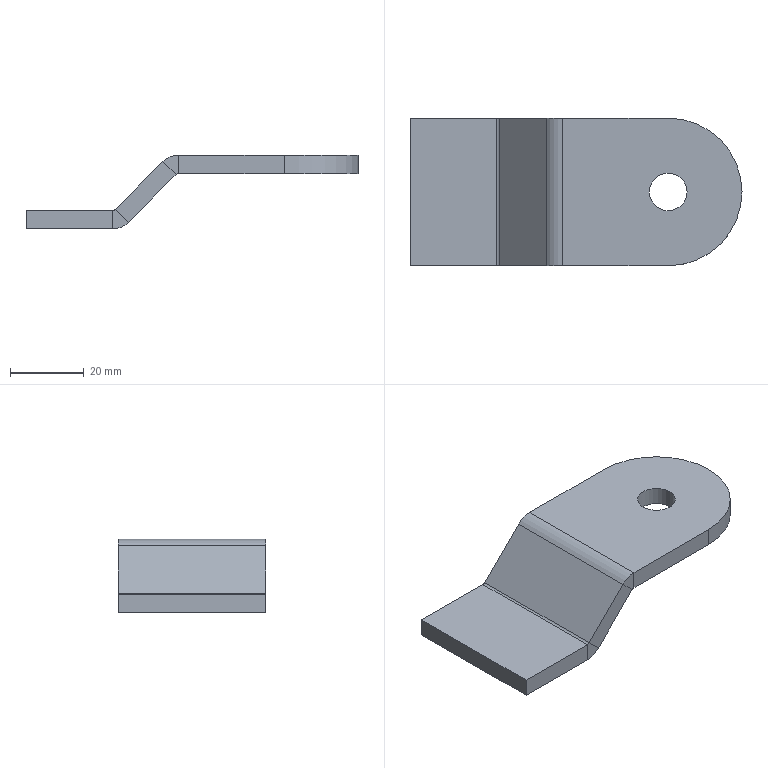Part | STEP file | 5090104 | 1 solid | 23 faces | box 90 x 40 x 20 mm | volume 17915 mm3 | plane 17 | cylinder 6 | commonest cylinder face diameters 2 x2 12 x2 10.2 x1 40 x1
STEP:
#1=CARTESIAN_POINT('',(0.,0.,0.));
#2=DIRECTION('',(0.,0.,1.));
#3=DIRECTION('',(1.,0.,0.));
#4=AXIS2_PLACEMENT_3D('',#1,#2,#3);
#5=CARTESIAN_POINT('',(-42.282,-20.,-13.243));
#6=VERTEX_POINT('',#5);
#7=CARTESIAN_POINT('',(-29.333,-20.,-0.2929));
#8=VERTEX_POINT('',#7);
#9=CARTESIAN_POINT('',(-56.645,-20.,-27.605));
#10=DIRECTION('',(0.7071,0.,0.7071));
#11=VECTOR('',#10,1.);
#12=LINE('',#9,#11);
#13=CARTESIAN_POINT('',(-7.148,0.,21.892));
#14=DIRECTION('',(0.7071,0.,-0.7071));
#15=DIRECTION('',(-0.7071,0.,-0.7071));
#16=AXIS2_PLACEMENT_3D('',#13,#14,#15);
#17=PLANE('',#16);
#18=CARTESIAN_POINT('',(70.,-20.));
#19=DIRECTION('',(-1.,0.));
#20=VECTOR('',#19,1.);
#21=LINE('',#18,#20);
#22=(GEOMETRIC_REPRESENTATION_CONTEXT(2)PARAMETRIC_REPRESENTATION_CONTEXT()REPRESENTATION_CONTEXT('',''));
#23=DEFINITIONAL_REPRESENTATION('',(#21),#22);
#24=PCURVE('',#17,#23);
#25=CARTESIAN_POINT('',(-60.181,-20.,-24.07));
#26=DIRECTION('',(0.,1.,0.));
#27=DIRECTION('',(-0.7071,0.,0.7071));
#28=AXIS2_PLACEMENT_3D('',#25,#26,#27);
#29=PLANE('',#28);
#30=CARTESIAN_POINT('',(-5.,0.));
#31=DIRECTION('',(0.,1.));
#32=VECTOR('',#31,1.);
#33=LINE('',#30,#32);
#34=(GEOMETRIC_REPRESENTATION_CONTEXT(2)PARAMETRIC_REPRESENTATION_CONTEXT()REPRESENTATION_CONTEXT('',''));
#35=DEFINITIONAL_REPRESENTATION('',(#33),#34);
#36=PCURVE('',#29,#35);
#37=SURFACE_CURVE('',#12,(#24,#36),.PCURVE_S1.);
#38=EDGE_CURVE('',#6,#8,#37,.T.);
#39=ORIENTED_EDGE('',*,*,#38,.F.);
#40=CARTESIAN_POINT('',(-42.282,20.,-13.243));
#41=VERTEX_POINT('',#40);
#42=CARTESIAN_POINT('',(-42.282,0.,-13.243));
#43=DIRECTION('',(0.,1.,0.));
#44=VECTOR('',#43,1.);
#45=LINE('',#42,#44);
#46=CARTESIAN_POINT('',(49.688,0.));
#47=DIRECTION('',(0.,1.));
#48=VECTOR('',#47,1.);
#49=LINE('',#46,#48);
#50=(GEOMETRIC_REPRESENTATION_CONTEXT(2)PARAMETRIC_REPRESENTATION_CONTEXT()REPRESENTATION_CONTEXT('',''));
#51=DEFINITIONAL_REPRESENTATION('',(#49),#50);
#52=PCURVE('',#17,#51);
#53=CARTESIAN_POINT('',(-46.525,40.744,-9.));
#54=DIRECTION('',(0.,-1.,0.));
#55=DIRECTION('',(1.,0.,0.));
#56=AXIS2_PLACEMENT_3D('',#53,#54,#55);
#57=CYLINDRICAL_SURFACE('',#56,6.);
#58=CARTESIAN_POINT('',(5.498,40.744));
#59=DIRECTION('',(0.,-1.));
#60=VECTOR('',#59,1.);
#61=LINE('',#58,#60);
#62=(GEOMETRIC_REPRESENTATION_CONTEXT(2)PARAMETRIC_REPRESENTATION_CONTEXT()REPRESENTATION_CONTEXT('',''));
#63=DEFINITIONAL_REPRESENTATION('',(#61),#62);
#64=PCURVE('',#57,#63);
#65=SURFACE_CURVE('',#45,(#52,#64),.PCURVE_S1.);
#66=EDGE_CURVE('',#6,#41,#65,.T.);
#67=ORIENTED_EDGE('',*,*,#66,.T.);
#68=CARTESIAN_POINT('',(-29.333,20.,-0.2929));
#69=VERTEX_POINT('',#68);
#70=CARTESIAN_POINT('',(-56.645,20.,-27.605));
#71=DIRECTION('',(-0.7071,0.,-0.7071));
#72=VECTOR('',#71,1.);
#73=LINE('',#70,#72);
#74=CARTESIAN_POINT('',(70.,20.));
#75=DIRECTION('',(1.,0.));
#76=VECTOR('',#75,1.);
#77=LINE('',#74,#76);
#78=(GEOMETRIC_REPRESENTATION_CONTEXT(2)PARAMETRIC_REPRESENTATION_CONTEXT()REPRESENTATION_CONTEXT('',''));
#79=DEFINITIONAL_REPRESENTATION('',(#77),#78);
#80=PCURVE('',#17,#79);
#81=CARTESIAN_POINT('',(-60.181,20.,-24.07));
#82=DIRECTION('',(0.,-1.,0.));
#83=DIRECTION('',(0.7071,0.,-0.7071));
#84=AXIS2_PLACEMENT_3D('',#81,#82,#83);
#85=PLANE('',#84);
#86=CARTESIAN_POINT('',(5.,0.));
#87=DIRECTION('',(0.,-1.));
#88=VECTOR('',#87,1.);
#89=LINE('',#86,#88);
#90=(GEOMETRIC_REPRESENTATION_CONTEXT(2)PARAMETRIC_REPRESENTATION_CONTEXT()REPRESENTATION_CONTEXT('',''));
#91=DEFINITIONAL_REPRESENTATION('',(#89),#90);
#92=PCURVE('',#85,#91);
#93=SURFACE_CURVE('',#73,(#80,#92),.PCURVE_S1.);
#94=EDGE_CURVE('',#69,#41,#93,.T.);
#95=ORIENTED_EDGE('',*,*,#94,.F.);
#96=CARTESIAN_POINT('',(-29.333,0.,-0.2929));
#97=DIRECTION('',(0.,1.,0.));
#98=VECTOR('',#97,1.);
#99=LINE('',#96,#98);
#100=CARTESIAN_POINT('',(31.374,0.));
#101=DIRECTION('',(0.,1.));
#102=VECTOR('',#101,1.);
#103=LINE('',#100,#102);
#104=(GEOMETRIC_REPRESENTATION_CONTEXT(2)PARAMETRIC_REPRESENTATION_CONTEXT()REPRESENTATION_CONTEXT('',''));
#105=DEFINITIONAL_REPRESENTATION('',(#103),#104);
#106=PCURVE('',#17,#105);
#107=CARTESIAN_POINT('',(-28.626,40.405,-1.));
#108=DIRECTION('',(0.,-1.,0.));
#109=DIRECTION('',(1.,0.,0.));
#110=AXIS2_PLACEMENT_3D('',#107,#108,#109);
#111=CYLINDRICAL_SURFACE('',#110,1.);
#112=CARTESIAN_POINT('',(2.356,40.405));
#113=DIRECTION('',(0.,-1.));
#114=VECTOR('',#113,1.);
#115=LINE('',#112,#114);
#116=(GEOMETRIC_REPRESENTATION_CONTEXT(2)PARAMETRIC_REPRESENTATION_CONTEXT()REPRESENTATION_CONTEXT('',''));
#117=DEFINITIONAL_REPRESENTATION('',(#115),#116);
#118=PCURVE('',#111,#117);
#119=SURFACE_CURVE('',#99,(#106,#118),.PCURVE_S1.);
#120=EDGE_CURVE('',#8,#69,#119,.T.);
#121=ORIENTED_EDGE('',*,*,#120,.F.);
#122=EDGE_LOOP('',(#39,#67,#95,#121));
#123=FACE_BOUND('',#122,.T.);
#124=ADVANCED_FACE('',(#123),#17,.T.);
#125=CARTESIAN_POINT('',(-45.818,20.,-9.707));
#126=VERTEX_POINT('',#125);
#127=CARTESIAN_POINT('',(-45.818,20.,-9.707));
#128=DIRECTION('',(0.7071,0.,-0.7071));
#129=VECTOR('',#128,1.);
#130=LINE('',#127,#129);
#131=CARTESIAN_POINT('',(0.,20.312));
#132=DIRECTION('',(1.,0.));
#133=VECTOR('',#132,1.);
#134=LINE('',#131,#133);
#135=(GEOMETRIC_REPRESENTATION_CONTEXT(2)PARAMETRIC_REPRESENTATION_CONTEXT()REPRESENTATION_CONTEXT('',''));
#136=DEFINITIONAL_REPRESENTATION('',(#134),#135);
#137=PCURVE('',#85,#136);
#138=CARTESIAN_POINT('',(-46.525,20.,-9.));
#139=DIRECTION('',(0.,-1.,0.));
#140=DIRECTION('',(0.,0.,-1.));
#141=AXIS2_PLACEMENT_3D('',#138,#139,#140);
#142=PLANE('',#141);
#143=CARTESIAN_POINT('',(0.7071,0.7071));
#144=DIRECTION('',(0.7071,0.7071));
#145=VECTOR('',#144,1.);
#146=LINE('',#143,#145);
#147=(GEOMETRIC_REPRESENTATION_CONTEXT(2)PARAMETRIC_REPRESENTATION_CONTEXT()REPRESENTATION_CONTEXT('',''));
#148=DEFINITIONAL_REPRESENTATION('',(#146),#147);
#149=PCURVE('',#142,#148);
#150=SURFACE_CURVE('',#130,(#137,#149),.PCURVE_S1.);
#151=EDGE_CURVE('',#126,#41,#150,.T.);
#152=ORIENTED_EDGE('',*,*,#151,.F.);
#153=CARTESIAN_POINT('',(-32.868,20.,3.243));
#154=VERTEX_POINT('',#153);
#155=CARTESIAN_POINT('',(-60.181,20.,-24.07));
#156=DIRECTION('',(-0.7071,0.,-0.7071));
#157=VECTOR('',#156,1.);
#158=LINE('',#155,#157);
#159=CARTESIAN_POINT('',(0.,0.));
#160=DIRECTION('',(0.,-1.));
#161=VECTOR('',#160,1.);
#162=LINE('',#159,#161);
#163=(GEOMETRIC_REPRESENTATION_CONTEXT(2)PARAMETRIC_REPRESENTATION_CONTEXT()REPRESENTATION_CONTEXT('',''));
#164=DEFINITIONAL_REPRESENTATION('',(#162),#163);
#165=PCURVE('',#85,#164);
#166=CARTESIAN_POINT('',(-10.683,0.,25.428));
#167=DIRECTION('',(0.7071,0.,-0.7071));
#168=DIRECTION('',(-0.7071,0.,-0.7071));
#169=AXIS2_PLACEMENT_3D('',#166,#167,#168);
#170=PLANE('',#169);
#171=CARTESIAN_POINT('',(70.,20.));
#172=DIRECTION('',(1.,0.));
#173=VECTOR('',#172,1.);
#174=LINE('',#171,#173);
#175=(GEOMETRIC_REPRESENTATION_CONTEXT(2)PARAMETRIC_REPRESENTATION_CONTEXT()REPRESENTATION_CONTEXT('',''));
#176=DEFINITIONAL_REPRESENTATION('',(#174),#175);
#177=PCURVE('',#170,#176);
#178=SURFACE_CURVE('',#158,(#165,#177),.PCURVE_S1.);
#179=EDGE_CURVE('',#154,#126,#178,.T.);
#180=ORIENTED_EDGE('',*,*,#179,.F.);
#181=CARTESIAN_POINT('',(-32.868,20.,3.243));
#182=DIRECTION('',(0.7071,0.,-0.7071));
#183=VECTOR('',#182,1.);
#184=LINE('',#181,#183);
#185=CARTESIAN_POINT('',(0.,38.626));
#186=DIRECTION('',(1.,0.));
#187=VECTOR('',#186,1.);
#188=LINE('',#185,#187);
#189=(GEOMETRIC_REPRESENTATION_CONTEXT(2)PARAMETRIC_REPRESENTATION_CONTEXT()REPRESENTATION_CONTEXT('',''));
#190=DEFINITIONAL_REPRESENTATION('',(#188),#189);
#191=PCURVE('',#85,#190);
#192=CARTESIAN_POINT('',(-28.626,20.,-1.));
#193=DIRECTION('',(0.,1.,0.));
#194=DIRECTION('',(0.,0.,1.));
#195=AXIS2_PLACEMENT_3D('',#192,#193,#194);
#196=PLANE('',#195);
#197=CARTESIAN_POINT('',(4.243,-4.243));
#198=DIRECTION('',(-0.7071,0.7071));
#199=VECTOR('',#198,1.);
#200=LINE('',#197,#199);
#201=(GEOMETRIC_REPRESENTATION_CONTEXT(2)PARAMETRIC_REPRESENTATION_CONTEXT()REPRESENTATION_CONTEXT('',''));
#202=DEFINITIONAL_REPRESENTATION('',(#200),#201);
#203=PCURVE('',#196,#202);
#204=SURFACE_CURVE('',#184,(#191,#203),.PCURVE_S1.);
#205=EDGE_CURVE('',#154,#69,#204,.T.);
#206=ORIENTED_EDGE('',*,*,#205,.T.);
#207=ORIENTED_EDGE('',*,*,#94,.T.);
#208=EDGE_LOOP('',(#152,#180,#206,#207));
#209=FACE_BOUND('',#208,.T.);
#210=ADVANCED_FACE('',(#209),#85,.F.);
#211=CARTESIAN_POINT('',(-45.818,-20.,-9.707));
#212=VERTEX_POINT('',#211);
#213=CARTESIAN_POINT('',(-45.818,-20.,-9.707));
#214=DIRECTION('',(-0.7071,0.,0.7071));
#215=VECTOR('',#214,1.);
#216=LINE('',#213,#215);
#217=CARTESIAN_POINT('',(0.,20.312));
#218=DIRECTION('',(1.,0.));
#219=VECTOR('',#218,1.);
#220=LINE('',#217,#219);
#221=(GEOMETRIC_REPRESENTATION_CONTEXT(2)PARAMETRIC_REPRESENTATION_CONTEXT()REPRESENTATION_CONTEXT('',''));
#222=DEFINITIONAL_REPRESENTATION('',(#220),#221);
#223=PCURVE('',#29,#222);
#224=CARTESIAN_POINT('',(-46.525,-20.,-9.));
#225=DIRECTION('',(0.,1.,0.));
#226=DIRECTION('',(0.,0.,1.));
#227=AXIS2_PLACEMENT_3D('',#224,#225,#226);
#228=PLANE('',#227);
#229=CARTESIAN_POINT('',(-0.7071,0.7071));
#230=DIRECTION('',(0.7071,-0.7071));
#231=VECTOR('',#230,1.);
#232=LINE('',#229,#231);
#233=(GEOMETRIC_REPRESENTATION_CONTEXT(2)PARAMETRIC_REPRESENTATION_CONTEXT()REPRESENTATION_CONTEXT('',''));
#234=DEFINITIONAL_REPRESENTATION('',(#232),#233);
#235=PCURVE('',#228,#234);
#236=SURFACE_CURVE('',#216,(#223,#235),.PCURVE_S1.);
#237=EDGE_CURVE('',#6,#212,#236,.T.);
#238=ORIENTED_EDGE('',*,*,#237,.F.);
#239=ORIENTED_EDGE('',*,*,#38,.T.);
#240=CARTESIAN_POINT('',(-32.868,-20.,3.243));
#241=VERTEX_POINT('',#240);
#242=CARTESIAN_POINT('',(-32.868,-20.,3.243));
#243=DIRECTION('',(-0.7071,0.,0.7071));
#244=VECTOR('',#243,1.);
#245=LINE('',#242,#244);
#246=CARTESIAN_POINT('',(0.,38.626));
#247=DIRECTION('',(1.,0.));
#248=VECTOR('',#247,1.);
#249=LINE('',#246,#248);
#250=(GEOMETRIC_REPRESENTATION_CONTEXT(2)PARAMETRIC_REPRESENTATION_CONTEXT()REPRESENTATION_CONTEXT('',''));
#251=DEFINITIONAL_REPRESENTATION('',(#249),#250);
#252=PCURVE('',#29,#251);
#253=CARTESIAN_POINT('',(-28.626,-20.,-1.));
#254=DIRECTION('',(0.,-1.,0.));
#255=DIRECTION('',(0.,0.,-1.));
#256=AXIS2_PLACEMENT_3D('',#253,#254,#255);
#257=PLANE('',#256);
#258=CARTESIAN_POINT('',(-4.243,-4.243));
#259=DIRECTION('',(-0.7071,-0.7071));
#260=VECTOR('',#259,1.);
#261=LINE('',#258,#260);
#262=(GEOMETRIC_REPRESENTATION_CONTEXT(2)PARAMETRIC_REPRESENTATION_CONTEXT()REPRESENTATION_CONTEXT('',''));
#263=DEFINITIONAL_REPRESENTATION('',(#261),#262);
#264=PCURVE('',#257,#263);
#265=SURFACE_CURVE('',#245,(#252,#264),.PCURVE_S1.);
#266=EDGE_CURVE('',#8,#241,#265,.T.);
#267=ORIENTED_EDGE('',*,*,#266,.T.);
#268=CARTESIAN_POINT('',(-60.181,-20.,-24.07));
#269=DIRECTION('',(0.7071,0.,0.7071));
#270=VECTOR('',#269,1.);
#271=LINE('',#268,#270);
#272=CARTESIAN_POINT('',(0.,0.));
#273=DIRECTION('',(0.,1.));
#274=VECTOR('',#273,1.);
#275=LINE('',#272,#274);
#276=(GEOMETRIC_REPRESENTATION_CONTEXT(2)PARAMETRIC_REPRESENTATION_CONTEXT()REPRESENTATION_CONTEXT('',''));
#277=DEFINITIONAL_REPRESENTATION('',(#275),#276);
#278=PCURVE('',#29,#277);
#279=CARTESIAN_POINT('',(70.,-20.));
#280=DIRECTION('',(-1.,0.));
#281=VECTOR('',#280,1.);
#282=LINE('',#279,#281);
#283=(GEOMETRIC_REPRESENTATION_CONTEXT(2)PARAMETRIC_REPRESENTATION_CONTEXT()REPRESENTATION_CONTEXT('',''));
#284=DEFINITIONAL_REPRESENTATION('',(#282),#283);
#285=PCURVE('',#170,#284);
#286=SURFACE_CURVE('',#271,(#278,#285),.PCURVE_S1.);
#287=EDGE_CURVE('',#212,#241,#286,.T.);
#288=ORIENTED_EDGE('',*,*,#287,.F.);
#289=EDGE_LOOP('',(#238,#239,#267,#288));
#290=FACE_BOUND('',#289,.T.);
#291=ADVANCED_FACE('',(#290),#29,.F.);
#292=CARTESIAN_POINT('',(-45.818,0.,-9.707));
#293=DIRECTION('',(0.,1.,0.));
#294=VECTOR('',#293,1.);
#295=LINE('',#292,#294);
#296=CARTESIAN_POINT('',(49.688,0.));
#297=DIRECTION('',(0.,1.));
#298=VECTOR('',#297,1.);
#299=LINE('',#296,#298);
#300=(GEOMETRIC_REPRESENTATION_CONTEXT(2)PARAMETRIC_REPRESENTATION_CONTEXT()REPRESENTATION_CONTEXT('',''));
#301=DEFINITIONAL_REPRESENTATION('',(#299),#300);
#302=PCURVE('',#170,#301);
#303=CARTESIAN_POINT('',(-46.525,40.744,-9.));
#304=DIRECTION('',(0.,-1.,0.));
#305=DIRECTION('',(1.,0.,0.));
#306=AXIS2_PLACEMENT_3D('',#303,#304,#305);
#307=CYLINDRICAL_SURFACE('',#306,1.);
#308=CARTESIAN_POINT('',(5.498,40.744));
#309=DIRECTION('',(0.,-1.));
#310=VECTOR('',#309,1.);
#311=LINE('',#308,#310);
#312=(GEOMETRIC_REPRESENTATION_CONTEXT(2)PARAMETRIC_REPRESENTATION_CONTEXT()REPRESENTATION_CONTEXT('',''));
#313=DEFINITIONAL_REPRESENTATION('',(#311),#312);
#314=PCURVE('',#307,#313);
#315=SURFACE_CURVE('',#295,(#302,#314),.PCURVE_S1.);
#316=EDGE_CURVE('',#212,#126,#315,.T.);
#317=ORIENTED_EDGE('',*,*,#316,.F.);
#318=ORIENTED_EDGE('',*,*,#287,.T.);
#319=CARTESIAN_POINT('',(-32.868,0.,3.243));
#320=DIRECTION('',(0.,1.,0.));
#321=VECTOR('',#320,1.);
#322=LINE('',#319,#321);
#323=CARTESIAN_POINT('',(31.374,0.));
#324=DIRECTION('',(0.,1.));
#325=VECTOR('',#324,1.);
#326=LINE('',#323,#325);
#327=(GEOMETRIC_REPRESENTATION_CONTEXT(2)PARAMETRIC_REPRESENTATION_CONTEXT()REPRESENTATION_CONTEXT('',''));
#328=DEFINITIONAL_REPRESENTATION('',(#326),#327);
#329=PCURVE('',#170,#328);
#330=CARTESIAN_POINT('',(-28.626,40.405,-1.));
#331=DIRECTION('',(0.,-1.,0.));
#332=DIRECTION('',(1.,0.,0.));
#333=AXIS2_PLACEMENT_3D('',#330,#331,#332);
#334=CYLINDRICAL_SURFACE('',#333,6.);
#335=CARTESIAN_POINT('',(2.356,40.405));
#336=DIRECTION('',(0.,-1.));
#337=VECTOR('',#336,1.);
#338=LINE('',#335,#337);
#339=(GEOMETRIC_REPRESENTATION_CONTEXT(2)PARAMETRIC_REPRESENTATION_CONTEXT()REPRESENTATION_CONTEXT('',''));
#340=DEFINITIONAL_REPRESENTATION('',(#338),#339);
#341=PCURVE('',#334,#340);
#342=SURFACE_CURVE('',#322,(#329,#341),.PCURVE_S1.);
#343=EDGE_CURVE('',#241,#154,#342,.T.);
#344=ORIENTED_EDGE('',*,*,#343,.T.);
#345=ORIENTED_EDGE('',*,*,#179,.T.);
#346=EDGE_LOOP('',(#317,#318,#344,#345));
#347=FACE_BOUND('',#346,.T.);
#348=ADVANCED_FACE('',(#347),#170,.F.);
#349=CARTESIAN_POINT('',(5.1,0.,5.));
#350=VERTEX_POINT('',#349);
#351=CARTESIAN_POINT('',(0.,0.,5.));
#352=DIRECTION('',(0.,0.,1.));
#353=DIRECTION('',(1.,0.,0.));
#354=AXIS2_PLACEMENT_3D('',#351,#352,#353);
#355=CIRCLE('',#354,5.1);
#356=CARTESIAN_POINT('',(0.,0.,5.));
#357=DIRECTION('',(0.,0.,-1.));
#358=DIRECTION('',(-1.,0.,0.));
#359=AXIS2_PLACEMENT_3D('',#356,#357,#358);
#360=CYLINDRICAL_SURFACE('',#359,5.1);
#361=CARTESIAN_POINT('',(9.425,0.));
#362=DIRECTION('',(-1.,0.));
#363=VECTOR('',#362,1.);
#364=LINE('',#361,#363);
#365=(GEOMETRIC_REPRESENTATION_CONTEXT(2)PARAMETRIC_REPRESENTATION_CONTEXT()REPRESENTATION_CONTEXT('',''));
#366=DEFINITIONAL_REPRESENTATION('',(#364),#365);
#367=PCURVE('',#360,#366);
#368=CARTESIAN_POINT('',(0.,0.,5.));
#369=DIRECTION('',(0.,0.,-1.));
#370=DIRECTION('',(-1.,0.,0.));
#371=AXIS2_PLACEMENT_3D('',#368,#369,#370);
#372=PLANE('',#371);
#373=CARTESIAN_POINT('',(-5.1,0.));
#374=CARTESIAN_POINT('',(-5.1,8.833));
#375=CARTESIAN_POINT('',(2.55,4.417));
#376=CARTESIAN_POINT('',(10.2,0.));
#377=CARTESIAN_POINT('',(2.55,-4.417));
#378=CARTESIAN_POINT('',(-5.1,-8.833));
#379=CARTESIAN_POINT('',(-5.1,0.));
#380=(BOUNDED_CURVE()B_SPLINE_CURVE(2,(#373,#374,#375,#376,#377,#378,#379),.UNSPECIFIED.,.T.,.F.)B_SPLINE_CURVE_WITH_KNOTS((1,2,2,2,2,1),(-2.094,0.,2.094,4.189,6.283,8.378),.UNSPECIFIED.)CURVE()GEOMETRIC_REPRESENTATION_ITEM()RATIONAL_B_SPLINE_CURVE((1.,0.5,1.,0.5,1.,0.5,1.))REPRESENTATION_ITEM(''));
#381=(GEOMETRIC_REPRESENTATION_CONTEXT(2)PARAMETRIC_REPRESENTATION_CONTEXT()REPRESENTATION_CONTEXT('',''));
#382=DEFINITIONAL_REPRESENTATION('',(#380),#381);
#383=PCURVE('',#372,#382);
#384=SURFACE_CURVE('',#355,(#367,#383),.PCURVE_S1.);
#385=EDGE_CURVE('',#350,#350,#384,.T.);
#386=ORIENTED_EDGE('',*,*,#385,.F.);
#387=CARTESIAN_POINT('',(5.1,0.,0.));
#388=VERTEX_POINT('',#387);
#389=CARTESIAN_POINT('',(5.1,0.,5.));
#390=CARTESIAN_POINT('',(5.1,0.,0.));
#391=B_SPLINE_CURVE_WITH_KNOTS('',1,(#389,#390),.UNSPECIFIED.,.F.,.F.,(2,2),(0.,5.),.PIECEWISE_BEZIER_KNOTS.);
#392=CARTESIAN_POINT('',(9.425,0.));
#393=DIRECTION('',(0.,1.));
#394=VECTOR('',#393,1.);
#395=LINE('',#392,#394);
#396=(GEOMETRIC_REPRESENTATION_CONTEXT(2)PARAMETRIC_REPRESENTATION_CONTEXT()REPRESENTATION_CONTEXT('',''));
#397=DEFINITIONAL_REPRESENTATION('',(#395),#396);
#398=PCURVE('',#360,#397);
#399=CARTESIAN_POINT('',(3.142,0.));
#400=DIRECTION('',(0.,1.));
#401=VECTOR('',#400,1.);
#402=LINE('',#399,#401);
#403=(GEOMETRIC_REPRESENTATION_CONTEXT(2)PARAMETRIC_REPRESENTATION_CONTEXT()REPRESENTATION_CONTEXT('',''));
#404=DEFINITIONAL_REPRESENTATION('',(#402),#403);
#405=PCURVE('',#360,#404);
#406=SEAM_CURVE('',#391,(#398,#405),.PCURVE_S1.);
#407=EDGE_CURVE('',#350,#388,#406,.T.);
#408=ORIENTED_EDGE('',*,*,#407,.T.);
#409=CARTESIAN_POINT('',(0.,0.,0.));
#410=DIRECTION('',(0.,0.,1.));
#411=DIRECTION('',(1.,0.,0.));
#412=AXIS2_PLACEMENT_3D('',#409,#410,#411);
#413=CIRCLE('',#412,5.1);
#414=CARTESIAN_POINT('',(9.425,5.));
#415=DIRECTION('',(-1.,0.));
#416=VECTOR('',#415,1.);
#417=LINE('',#414,#416);
#418=(GEOMETRIC_REPRESENTATION_CONTEXT(2)PARAMETRIC_REPRESENTATION_CONTEXT()REPRESENTATION_CONTEXT('',''));
#419=DEFINITIONAL_REPRESENTATION('',(#417),#418);
#420=PCURVE('',#360,#419);
#421=CARTESIAN_POINT('',(0.,0.,0.));
#422=DIRECTION('',(0.,0.,-1.));
#423=DIRECTION('',(-1.,0.,0.));
#424=AXIS2_PLACEMENT_3D('',#421,#422,#423);
#425=PLANE('',#424);
#426=CARTESIAN_POINT('',(-5.1,0.));
#427=CARTESIAN_POINT('',(-5.1,8.833));
#428=CARTESIAN_POINT('',(2.55,4.417));
#429=CARTESIAN_POINT('',(10.2,0.));
#430=CARTESIAN_POINT('',(2.55,-4.417));
#431=CARTESIAN_POINT('',(-5.1,-8.833));
#432=CARTESIAN_POINT('',(-5.1,0.));
#433=(BOUNDED_CURVE()B_SPLINE_CURVE(2,(#426,#427,#428,#429,#430,#431,#432),.UNSPECIFIED.,.T.,.F.)B_SPLINE_CURVE_WITH_KNOTS((1,2,2,2,2,1),(-2.094,0.,2.094,4.189,6.283,8.378),.UNSPECIFIED.)CURVE()GEOMETRIC_REPRESENTATION_ITEM()RATIONAL_B_SPLINE_CURVE((1.,0.5,1.,0.5,1.,0.5,1.))REPRESENTATION_ITEM(''));
#434=(GEOMETRIC_REPRESENTATION_CONTEXT(2)PARAMETRIC_REPRESENTATION_CONTEXT()REPRESENTATION_CONTEXT('',''));
#435=DEFINITIONAL_REPRESENTATION('',(#433),#434);
#436=PCURVE('',#425,#435);
#437=SURFACE_CURVE('',#413,(#420,#436),.PCURVE_S1.);
#438=EDGE_CURVE('',#388,#388,#437,.T.);
#439=ORIENTED_EDGE('',*,*,#438,.T.);
#440=ORIENTED_EDGE('',*,*,#407,.F.);
#441=EDGE_LOOP('',(#386,#408,#439,#440));
#442=FACE_BOUND('',#441,.F.);
#443=ADVANCED_FACE('',(#442),#360,.F.);
#444=CARTESIAN_POINT('',(0.,-20.,0.));
#445=VERTEX_POINT('',#444);
#446=CARTESIAN_POINT('',(0.,20.,0.));
#447=VERTEX_POINT('',#446);
#448=CARTESIAN_POINT('',(0.,0.,0.));
#449=DIRECTION('',(0.,0.,1.));
#450=DIRECTION('',(-1.,0.,0.));
#451=AXIS2_PLACEMENT_3D('',#448,#449,#450);
#452=CIRCLE('',#451,20.);
#453=CARTESIAN_POINT('',(0.,0.,5.));
#454=DIRECTION('',(0.,0.,-1.));
#455=DIRECTION('',(-1.,0.,0.));
#456=AXIS2_PLACEMENT_3D('',#453,#454,#455);
#457=CYLINDRICAL_SURFACE('',#456,20.);
#458=CARTESIAN_POINT('',(6.283,5.));
#459=DIRECTION('',(-1.,0.));
#460=VECTOR('',#459,1.);
#461=LINE('',#458,#460);
#462=(GEOMETRIC_REPRESENTATION_CONTEXT(2)PARAMETRIC_REPRESENTATION_CONTEXT()REPRESENTATION_CONTEXT('',''));
#463=DEFINITIONAL_REPRESENTATION('',(#461),#462);
#464=PCURVE('',#457,#463);
#465=CARTESIAN_POINT('',(20.,0.));
#466=CARTESIAN_POINT('',(20.,-34.641));
#467=CARTESIAN_POINT('',(-10.,-17.321));
#468=CARTESIAN_POINT('',(-40.,0.));
#469=CARTESIAN_POINT('',(-10.,17.321));
#470=CARTESIAN_POINT('',(20.,34.641));
#471=CARTESIAN_POINT('',(20.,0.));
#472=(BOUNDED_CURVE()B_SPLINE_CURVE(2,(#465,#466,#467,#468,#469,#470,#471),.UNSPECIFIED.,.T.,.F.)B_SPLINE_CURVE_WITH_KNOTS((1,2,2,2,2,1),(-2.094,0.,2.094,4.189,6.283,8.378),.UNSPECIFIED.)CURVE()GEOMETRIC_REPRESENTATION_ITEM()RATIONAL_B_SPLINE_CURVE((1.,0.5,1.,0.5,1.,0.5,1.))REPRESENTATION_ITEM(''));
#473=(GEOMETRIC_REPRESENTATION_CONTEXT(2)PARAMETRIC_REPRESENTATION_CONTEXT()REPRESENTATION_CONTEXT('',''));
#474=DEFINITIONAL_REPRESENTATION('',(#472),#473);
#475=PCURVE('',#425,#474);
#476=SURFACE_CURVE('',#452,(#464,#475),.PCURVE_S1.);
#477=EDGE_CURVE('',#445,#447,#476,.T.);
#478=ORIENTED_EDGE('',*,*,#477,.T.);
#479=CARTESIAN_POINT('',(0.,20.,5.));
#480=VERTEX_POINT('',#479);
#481=CARTESIAN_POINT('',(0.,20.,5.));
#482=DIRECTION('',(0.,0.,-1.));
#483=VECTOR('',#482,1.);
#484=LINE('',#481,#483);
#485=CARTESIAN_POINT('',(1.571,0.));
#486=DIRECTION('',(0.,1.));
#487=VECTOR('',#486,1.);
#488=LINE('',#485,#487);
#489=(GEOMETRIC_REPRESENTATION_CONTEXT(2)PARAMETRIC_REPRESENTATION_CONTEXT()REPRESENTATION_CONTEXT('',''));
#490=DEFINITIONAL_REPRESENTATION('',(#488),#489);
#491=PCURVE('',#457,#490);
#492=CARTESIAN_POINT('',(-70.,20.,5.));
#493=DIRECTION('',(0.,-1.,0.));
#494=DIRECTION('',(0.,0.,-1.));
#495=AXIS2_PLACEMENT_3D('',#492,#493,#494);
#496=PLANE('',#495);
#497=CARTESIAN_POINT('',(0.,70.));
#498=DIRECTION('',(1.,0.));
#499=VECTOR('',#498,1.);
#500=LINE('',#497,#499);
#501=(GEOMETRIC_REPRESENTATION_CONTEXT(2)PARAMETRIC_REPRESENTATION_CONTEXT()REPRESENTATION_CONTEXT('',''));
#502=DEFINITIONAL_REPRESENTATION('',(#500),#501);
#503=PCURVE('',#496,#502);
#504=SURFACE_CURVE('',#484,(#491,#503),.PCURVE_S1.);
#505=EDGE_CURVE('',#480,#447,#504,.T.);
#506=ORIENTED_EDGE('',*,*,#505,.F.);
#507=CARTESIAN_POINT('',(0.,-20.,5.));
#508=VERTEX_POINT('',#507);
#509=CARTESIAN_POINT('',(0.,0.,5.));
#510=DIRECTION('',(0.,0.,1.));
#511=DIRECTION('',(-1.,0.,0.));
#512=AXIS2_PLACEMENT_3D('',#509,#510,#511);
#513=CIRCLE('',#512,20.);
#514=CARTESIAN_POINT('',(6.283,0.));
#515=DIRECTION('',(-1.,0.));
#516=VECTOR('',#515,1.);
#517=LINE('',#514,#516);
#518=(GEOMETRIC_REPRESENTATION_CONTEXT(2)PARAMETRIC_REPRESENTATION_CONTEXT()REPRESENTATION_CONTEXT('',''));
#519=DEFINITIONAL_REPRESENTATION('',(#517),#518);
#520=PCURVE('',#457,#519);
#521=CARTESIAN_POINT('',(20.,0.));
#522=CARTESIAN_POINT('',(20.,-34.641));
#523=CARTESIAN_POINT('',(-10.,-17.321));
#524=CARTESIAN_POINT('',(-40.,0.));
#525=CARTESIAN_POINT('',(-10.,17.321));
#526=CARTESIAN_POINT('',(20.,34.641));
#527=CARTESIAN_POINT('',(20.,0.));
#528=(BOUNDED_CURVE()B_SPLINE_CURVE(2,(#521,#522,#523,#524,#525,#526,#527),.UNSPECIFIED.,.T.,.F.)B_SPLINE_CURVE_WITH_KNOTS((1,2,2,2,2,1),(-2.094,0.,2.094,4.189,6.283,8.378),.UNSPECIFIED.)CURVE()GEOMETRIC_REPRESENTATION_ITEM()RATIONAL_B_SPLINE_CURVE((1.,0.5,1.,0.5,1.,0.5,1.))REPRESENTATION_ITEM(''));
#529=(GEOMETRIC_REPRESENTATION_CONTEXT(2)PARAMETRIC_REPRESENTATION_CONTEXT()REPRESENTATION_CONTEXT('',''));
#530=DEFINITIONAL_REPRESENTATION('',(#528),#529);
#531=PCURVE('',#372,#530);
#532=SURFACE_CURVE('',#513,(#520,#531),.PCURVE_S1.);
#533=EDGE_CURVE('',#508,#480,#532,.T.);
#534=ORIENTED_EDGE('',*,*,#533,.F.);
#535=CARTESIAN_POINT('',(0.,-20.,5.));
#536=DIRECTION('',(0.,0.,-1.));
#537=VECTOR('',#536,1.);
#538=LINE('',#535,#537);
#539=CARTESIAN_POINT('',(4.712,0.));
#540=DIRECTION('',(0.,1.));
#541=VECTOR('',#540,1.);
#542=LINE('',#539,#541);
#543=(GEOMETRIC_REPRESENTATION_CONTEXT(2)PARAMETRIC_REPRESENTATION_CONTEXT()REPRESENTATION_CONTEXT('',''));
#544=DEFINITIONAL_REPRESENTATION('',(#542),#543);
#545=PCURVE('',#457,#544);
#546=CARTESIAN_POINT('',(-70.,-20.,5.));
#547=DIRECTION('',(0.,1.,0.));
#548=DIRECTION('',(0.,0.,1.));
#549=AXIS2_PLACEMENT_3D('',#546,#547,#548);
#550=PLANE('',#549);
#551=CARTESIAN_POINT('',(0.,70.));
#552=DIRECTION('',(-1.,0.));
#553=VECTOR('',#552,1.);
#554=LINE('',#551,#553);
#555=(GEOMETRIC_REPRESENTATION_CONTEXT(2)PARAMETRIC_REPRESENTATION_CONTEXT()REPRESENTATION_CONTEXT('',''));
#556=DEFINITIONAL_REPRESENTATION('',(#554),#555);
#557=PCURVE('',#550,#556);
#558=SURFACE_CURVE('',#538,(#545,#557),.PCURVE_S1.);
#559=EDGE_CURVE('',#508,#445,#558,.T.);
#560=ORIENTED_EDGE('',*,*,#559,.T.);
#561=EDGE_LOOP('',(#478,#506,#534,#560));
#562=FACE_BOUND('',#561,.T.);
#563=ADVANCED_FACE('',(#562),#457,.T.);
#564=CARTESIAN_POINT('',(-28.626,-20.,5.));
#565=VERTEX_POINT('',#564);
#566=CARTESIAN_POINT('',(-28.626,20.,5.));
#567=VERTEX_POINT('',#566);
#568=CARTESIAN_POINT('',(-28.626,0.,5.));
#569=DIRECTION('',(0.,1.,0.));
#570=VECTOR('',#569,1.);
#571=LINE('',#568,#570);
#572=CARTESIAN_POINT('',(28.626,0.));
#573=DIRECTION('',(0.,1.));
#574=VECTOR('',#573,1.);
#575=LINE('',#572,#574);
#576=(GEOMETRIC_REPRESENTATION_CONTEXT(2)PARAMETRIC_REPRESENTATION_CONTEXT()REPRESENTATION_CONTEXT('',''));
#577=DEFINITIONAL_REPRESENTATION('',(#575),#576);
#578=PCURVE('',#372,#577);
#579=CARTESIAN_POINT('',(1.571,40.405));
#580=DIRECTION('',(0.,-1.));
#581=VECTOR('',#580,1.);
#582=LINE('',#579,#581);
#583=(GEOMETRIC_REPRESENTATION_CONTEXT(2)PARAMETRIC_REPRESENTATION_CONTEXT()REPRESENTATION_CONTEXT('',''));
#584=DEFINITIONAL_REPRESENTATION('',(#582),#583);
#585=PCURVE('',#334,#584);
#586=SURFACE_CURVE('',#571,(#578,#585),.PCURVE_S1.);
#587=EDGE_CURVE('',#565,#567,#586,.T.);
#588=ORIENTED_EDGE('',*,*,#587,.F.);
#589=CARTESIAN_POINT('',(-70.,-20.,5.));
#590=DIRECTION('',(1.,0.,0.));
#591=VECTOR('',#590,1.);
#592=LINE('',#589,#591);
#593=CARTESIAN_POINT('',(70.,-20.));
#594=DIRECTION('',(-1.,0.));
#595=VECTOR('',#594,1.);
#596=LINE('',#593,#595);
#597=(GEOMETRIC_REPRESENTATION_CONTEXT(2)PARAMETRIC_REPRESENTATION_CONTEXT()REPRESENTATION_CONTEXT('',''));
#598=DEFINITIONAL_REPRESENTATION('',(#596),#597);
#599=PCURVE('',#372,#598);
#600=CARTESIAN_POINT('',(0.,0.));
#601=DIRECTION('',(0.,1.));
#602=VECTOR('',#601,1.);
#603=LINE('',#600,#602);
#604=(GEOMETRIC_REPRESENTATION_CONTEXT(2)PARAMETRIC_REPRESENTATION_CONTEXT()REPRESENTATION_CONTEXT('',''));
#605=DEFINITIONAL_REPRESENTATION('',(#603),#604);
#606=PCURVE('',#550,#605);
#607=SURFACE_CURVE('',#592,(#599,#606),.PCURVE_S1.);
#608=EDGE_CURVE('',#565,#508,#607,.T.);
#609=ORIENTED_EDGE('',*,*,#608,.T.);
#610=ORIENTED_EDGE('',*,*,#533,.T.);
#611=CARTESIAN_POINT('',(-70.,20.,5.));
#612=DIRECTION('',(-1.,0.,0.));
#613=VECTOR('',#612,1.);
#614=LINE('',#611,#613);
#615=CARTESIAN_POINT('',(70.,20.));
#616=DIRECTION('',(1.,0.));
#617=VECTOR('',#616,1.);
#618=LINE('',#615,#617);
#619=(GEOMETRIC_REPRESENTATION_CONTEXT(2)PARAMETRIC_REPRESENTATION_CONTEXT()REPRESENTATION_CONTEXT('',''));
#620=DEFINITIONAL_REPRESENTATION('',(#618),#619);
#621=PCURVE('',#372,#620);
#622=CARTESIAN_POINT('',(0.,0.));
#623=DIRECTION('',(0.,-1.));
#624=VECTOR('',#623,1.);
#625=LINE('',#622,#624);
#626=(GEOMETRIC_REPRESENTATION_CONTEXT(2)PARAMETRIC_REPRESENTATION_CONTEXT()REPRESENTATION_CONTEXT('',''));
#627=DEFINITIONAL_REPRESENTATION('',(#625),#626);
#628=PCURVE('',#496,#627);
#629=SURFACE_CURVE('',#614,(#621,#628),.PCURVE_S1.);
#630=EDGE_CURVE('',#480,#567,#629,.T.);
#631=ORIENTED_EDGE('',*,*,#630,.T.);
#632=EDGE_LOOP('',(#588,#609,#610,#631));
#633=FACE_BOUND('',#632,.T.);
#634=ORIENTED_EDGE('',*,*,#385,.F.);
#635=EDGE_LOOP('',(#634));
#636=FACE_BOUND('',#635,.T.);
#637=ADVANCED_FACE('',(#633,#636),#372,.F.);
#638=CARTESIAN_POINT('',(-28.626,-20.,0.));
#639=VERTEX_POINT('',#638);
#640=CARTESIAN_POINT('',(-28.626,-20.,5.));
#641=DIRECTION('',(0.,0.,1.));
#642=VECTOR('',#641,1.);
#643=LINE('',#640,#642);
#644=CARTESIAN_POINT('',(0.,41.374));
#645=DIRECTION('',(1.,0.));
#646=VECTOR('',#645,1.);
#647=LINE('',#644,#646);
#648=(GEOMETRIC_REPRESENTATION_CONTEXT(2)PARAMETRIC_REPRESENTATION_CONTEXT()REPRESENTATION_CONTEXT('',''));
#649=DEFINITIONAL_REPRESENTATION('',(#647),#648);
#650=PCURVE('',#550,#649);
#651=CARTESIAN_POINT('',(-6.,0.));
#652=DIRECTION('',(-1.,0.));
#653=VECTOR('',#652,1.);
#654=LINE('',#651,#653);
#655=(GEOMETRIC_REPRESENTATION_CONTEXT(2)PARAMETRIC_REPRESENTATION_CONTEXT()REPRESENTATION_CONTEXT('',''));
#656=DEFINITIONAL_REPRESENTATION('',(#654),#655);
#657=PCURVE('',#257,#656);
#658=SURFACE_CURVE('',#643,(#650,#657),.PCURVE_S1.);
#659=EDGE_CURVE('',#639,#565,#658,.T.);
#660=ORIENTED_EDGE('',*,*,#659,.F.);
#661=CARTESIAN_POINT('',(-70.,-20.,0.));
#662=DIRECTION('',(1.,0.,0.));
#663=VECTOR('',#662,1.);
#664=LINE('',#661,#663);
#665=CARTESIAN_POINT('',(-5.,0.));
#666=DIRECTION('',(0.,1.));
#667=VECTOR('',#666,1.);
#668=LINE('',#665,#667);
#669=(GEOMETRIC_REPRESENTATION_CONTEXT(2)PARAMETRIC_REPRESENTATION_CONTEXT()REPRESENTATION_CONTEXT('',''));
#670=DEFINITIONAL_REPRESENTATION('',(#668),#669);
#671=PCURVE('',#550,#670);
#672=CARTESIAN_POINT('',(70.,-20.));
#673=DIRECTION('',(-1.,0.));
#674=VECTOR('',#673,1.);
#675=LINE('',#672,#674);
#676=(GEOMETRIC_REPRESENTATION_CONTEXT(2)PARAMETRIC_REPRESENTATION_CONTEXT()REPRESENTATION_CONTEXT('',''));
#677=DEFINITIONAL_REPRESENTATION('',(#675),#676);
#678=PCURVE('',#425,#677);
#679=SURFACE_CURVE('',#664,(#671,#678),.PCURVE_S1.);
#680=EDGE_CURVE('',#639,#445,#679,.T.);
#681=ORIENTED_EDGE('',*,*,#680,.T.);
#682=ORIENTED_EDGE('',*,*,#559,.F.);
#683=ORIENTED_EDGE('',*,*,#608,.F.);
#684=EDGE_LOOP('',(#660,#681,#682,#683));
#685=FACE_BOUND('',#684,.T.);
#686=ADVANCED_FACE('',(#685),#550,.F.);
#687=ORIENTED_EDGE('',*,*,#438,.T.);
#688=EDGE_LOOP('',(#687));
#689=FACE_BOUND('',#688,.T.);
#690=ORIENTED_EDGE('',*,*,#680,.F.);
#691=CARTESIAN_POINT('',(-28.626,20.,0.));
#692=VERTEX_POINT('',#691);
#693=CARTESIAN_POINT('',(-28.626,0.,0.));
#694=DIRECTION('',(0.,1.,0.));
#695=VECTOR('',#694,1.);
#696=LINE('',#693,#695);
#697=CARTESIAN_POINT('',(28.626,0.));
#698=DIRECTION('',(0.,1.));
#699=VECTOR('',#698,1.);
#700=LINE('',#697,#699);
#701=(GEOMETRIC_REPRESENTATION_CONTEXT(2)PARAMETRIC_REPRESENTATION_CONTEXT()REPRESENTATION_CONTEXT('',''));
#702=DEFINITIONAL_REPRESENTATION('',(#700),#701);
#703=PCURVE('',#425,#702);
#704=CARTESIAN_POINT('',(1.571,40.405));
#705=DIRECTION('',(0.,-1.));
#706=VECTOR('',#705,1.);
#707=LINE('',#704,#706);
#708=(GEOMETRIC_REPRESENTATION_CONTEXT(2)PARAMETRIC_REPRESENTATION_CONTEXT()REPRESENTATION_CONTEXT('',''));
#709=DEFINITIONAL_REPRESENTATION('',(#707),#708);
#710=PCURVE('',#111,#709);
#711=SURFACE_CURVE('',#696,(#703,#710),.PCURVE_S1.);
#712=EDGE_CURVE('',#639,#692,#711,.T.);
#713=ORIENTED_EDGE('',*,*,#712,.T.);
#714=CARTESIAN_POINT('',(-70.,20.,0.));
#715=DIRECTION('',(-1.,0.,0.));
#716=VECTOR('',#715,1.);
#717=LINE('',#714,#716);
#718=CARTESIAN_POINT('',(70.,20.));
#719=DIRECTION('',(1.,0.));
#720=VECTOR('',#719,1.);
#721=LINE('',#718,#720);
#722=(GEOMETRIC_REPRESENTATION_CONTEXT(2)PARAMETRIC_REPRESENTATION_CONTEXT()REPRESENTATION_CONTEXT('',''));
#723=DEFINITIONAL_REPRESENTATION('',(#721),#722);
#724=PCURVE('',#425,#723);
#725=CARTESIAN_POINT('',(5.,0.));
#726=DIRECTION('',(0.,-1.));
#727=VECTOR('',#726,1.);
#728=LINE('',#725,#727);
#729=(GEOMETRIC_REPRESENTATION_CONTEXT(2)PARAMETRIC_REPRESENTATION_CONTEXT()REPRESENTATION_CONTEXT('',''));
#730=DEFINITIONAL_REPRESENTATION('',(#728),#729);
#731=PCURVE('',#496,#730);
#732=SURFACE_CURVE('',#717,(#724,#731),.PCURVE_S1.);
#733=EDGE_CURVE('',#447,#692,#732,.T.);
#734=ORIENTED_EDGE('',*,*,#733,.F.);
#735=ORIENTED_EDGE('',*,*,#477,.F.);
#736=EDGE_LOOP('',(#690,#713,#734,#735));
#737=FACE_BOUND('',#736,.T.);
#738=ADVANCED_FACE('',(#689,#737),#425,.T.);
#739=CARTESIAN_POINT('',(-28.626,20.,5.));
#740=DIRECTION('',(0.,0.,-1.));
#741=VECTOR('',#740,1.);
#742=LINE('',#739,#741);
#743=CARTESIAN_POINT('',(0.,41.374));
#744=DIRECTION('',(1.,0.));
#745=VECTOR('',#744,1.);
#746=LINE('',#743,#745);
#747=(GEOMETRIC_REPRESENTATION_CONTEXT(2)PARAMETRIC_REPRESENTATION_CONTEXT()REPRESENTATION_CONTEXT('',''));
#748=DEFINITIONAL_REPRESENTATION('',(#746),#747);
#749=PCURVE('',#496,#748);
#750=CARTESIAN_POINT('',(6.,0.));
#751=DIRECTION('',(-1.,0.));
#752=VECTOR('',#751,1.);
#753=LINE('',#750,#752);
#754=(GEOMETRIC_REPRESENTATION_CONTEXT(2)PARAMETRIC_REPRESENTATION_CONTEXT()REPRESENTATION_CONTEXT('',''));
#755=DEFINITIONAL_REPRESENTATION('',(#753),#754);
#756=PCURVE('',#196,#755);
#757=SURFACE_CURVE('',#742,(#749,#756),.PCURVE_S1.);
#758=EDGE_CURVE('',#567,#692,#757,.T.);
#759=ORIENTED_EDGE('',*,*,#758,.F.);
#760=ORIENTED_EDGE('',*,*,#630,.F.);
#761=ORIENTED_EDGE('',*,*,#505,.T.);
#762=ORIENTED_EDGE('',*,*,#733,.T.);
#763=EDGE_LOOP('',(#759,#760,#761,#762));
#764=FACE_BOUND('',#763,.T.);
#765=ADVANCED_FACE('',(#764),#496,.F.);
#766=ORIENTED_EDGE('',*,*,#266,.F.);
#767=CARTESIAN_POINT('',(-28.626,-20.,-1.));
#768=DIRECTION('',(0.,1.,0.));
#769=DIRECTION('',(1.,0.,0.));
#770=AXIS2_PLACEMENT_3D('',#767,#768,#769);
#771=CIRCLE('',#770,1.);
#772=CARTESIAN_POINT('',(0.,1.));
#773=CARTESIAN_POINT('',(1.732,1.));
#774=CARTESIAN_POINT('',(0.866,-0.5));
#775=CARTESIAN_POINT('',(0.,-2.));
#776=CARTESIAN_POINT('',(-0.866,-0.5));
#777=CARTESIAN_POINT('',(-1.732,1.));
#778=CARTESIAN_POINT('',(0.,1.));
#779=(BOUNDED_CURVE()B_SPLINE_CURVE(2,(#772,#773,#774,#775,#776,#777,#778),.UNSPECIFIED.,.T.,.F.)B_SPLINE_CURVE_WITH_KNOTS((1,2,2,2,2,1),(-2.094,0.,2.094,4.189,6.283,8.378),.UNSPECIFIED.)CURVE()GEOMETRIC_REPRESENTATION_ITEM()RATIONAL_B_SPLINE_CURVE((1.,0.5,1.,0.5,1.,0.5,1.))REPRESENTATION_ITEM(''));
#780=(GEOMETRIC_REPRESENTATION_CONTEXT(2)PARAMETRIC_REPRESENTATION_CONTEXT()REPRESENTATION_CONTEXT('',''));
#781=DEFINITIONAL_REPRESENTATION('',(#779),#780);
#782=PCURVE('',#257,#781);
#783=CARTESIAN_POINT('',(6.283,60.405));
#784=DIRECTION('',(-1.,0.));
#785=VECTOR('',#784,1.);
#786=LINE('',#783,#785);
#787=(GEOMETRIC_REPRESENTATION_CONTEXT(2)PARAMETRIC_REPRESENTATION_CONTEXT()REPRESENTATION_CONTEXT('',''));
#788=DEFINITIONAL_REPRESENTATION('',(#786),#787);
#789=PCURVE('',#111,#788);
#790=SURFACE_CURVE('',#771,(#782,#789),.PCURVE_S1.);
#791=EDGE_CURVE('',#8,#639,#790,.T.);
#792=ORIENTED_EDGE('',*,*,#791,.T.);
#793=ORIENTED_EDGE('',*,*,#659,.T.);
#794=CARTESIAN_POINT('',(-28.626,-20.,-1.));
#795=DIRECTION('',(0.,1.,0.));
#796=DIRECTION('',(0.,0.,1.));
#797=AXIS2_PLACEMENT_3D('',#794,#795,#796);
#798=CIRCLE('',#797,6.);
#799=CARTESIAN_POINT('',(-6.,0.));
#800=CARTESIAN_POINT('',(-6.,10.392));
#801=CARTESIAN_POINT('',(3.,5.196));
#802=CARTESIAN_POINT('',(12.,0.));
#803=CARTESIAN_POINT('',(3.,-5.196));
#804=CARTESIAN_POINT('',(-6.,-10.392));
#805=CARTESIAN_POINT('',(-6.,0.));
#806=(BOUNDED_CURVE()B_SPLINE_CURVE(2,(#799,#800,#801,#802,#803,#804,#805),.UNSPECIFIED.,.T.,.F.)B_SPLINE_CURVE_WITH_KNOTS((1,2,2,2,2,1),(-2.094,0.,2.094,4.189,6.283,8.378),.UNSPECIFIED.)CURVE()GEOMETRIC_REPRESENTATION_ITEM()RATIONAL_B_SPLINE_CURVE((1.,0.5,1.,0.5,1.,0.5,1.))REPRESENTATION_ITEM(''));
#807=(GEOMETRIC_REPRESENTATION_CONTEXT(2)PARAMETRIC_REPRESENTATION_CONTEXT()REPRESENTATION_CONTEXT('',''));
#808=DEFINITIONAL_REPRESENTATION('',(#806),#807);
#809=PCURVE('',#257,#808);
#810=CARTESIAN_POINT('',(7.854,60.405));
#811=DIRECTION('',(-1.,0.));
#812=VECTOR('',#811,1.);
#813=LINE('',#810,#812);
#814=(GEOMETRIC_REPRESENTATION_CONTEXT(2)PARAMETRIC_REPRESENTATION_CONTEXT()REPRESENTATION_CONTEXT('',''));
#815=DEFINITIONAL_REPRESENTATION('',(#813),#814);
#816=PCURVE('',#334,#815);
#817=SURFACE_CURVE('',#798,(#809,#816),.PCURVE_S1.);
#818=EDGE_CURVE('',#241,#565,#817,.T.);
#819=ORIENTED_EDGE('',*,*,#818,.F.);
#820=EDGE_LOOP('',(#766,#792,#793,#819));
#821=FACE_BOUND('',#820,.T.);
#822=ADVANCED_FACE('',(#821),#257,.T.);
#823=ORIENTED_EDGE('',*,*,#758,.T.);
#824=CARTESIAN_POINT('',(-28.626,20.,-1.));
#825=DIRECTION('',(0.,-1.,0.));
#826=DIRECTION('',(1.,0.,0.));
#827=AXIS2_PLACEMENT_3D('',#824,#825,#826);
#828=CIRCLE('',#827,1.);
#829=CARTESIAN_POINT('',(0.,1.));
#830=CARTESIAN_POINT('',(1.732,1.));
#831=CARTESIAN_POINT('',(0.866,-0.5));
#832=CARTESIAN_POINT('',(0.,-2.));
#833=CARTESIAN_POINT('',(-0.866,-0.5));
#834=CARTESIAN_POINT('',(-1.732,1.));
#835=CARTESIAN_POINT('',(0.,1.));
#836=(BOUNDED_CURVE()B_SPLINE_CURVE(2,(#829,#830,#831,#832,#833,#834,#835),.UNSPECIFIED.,.T.,.F.)B_SPLINE_CURVE_WITH_KNOTS((1,2,2,2,2,1),(-2.094,0.,2.094,4.189,6.283,8.378),.UNSPECIFIED.)CURVE()GEOMETRIC_REPRESENTATION_ITEM()RATIONAL_B_SPLINE_CURVE((1.,0.5,1.,0.5,1.,0.5,1.))REPRESENTATION_ITEM(''));
#837=(GEOMETRIC_REPRESENTATION_CONTEXT(2)PARAMETRIC_REPRESENTATION_CONTEXT()REPRESENTATION_CONTEXT('',''));
#838=DEFINITIONAL_REPRESENTATION('',(#836),#837);
#839=PCURVE('',#196,#838);
#840=CARTESIAN_POINT('',(0.,20.405));
#841=DIRECTION('',(1.,0.));
#842=VECTOR('',#841,1.);
#843=LINE('',#840,#842);
#844=(GEOMETRIC_REPRESENTATION_CONTEXT(2)PARAMETRIC_REPRESENTATION_CONTEXT()REPRESENTATION_CONTEXT('',''));
#845=DEFINITIONAL_REPRESENTATION('',(#843),#844);
#846=PCURVE('',#111,#845);
#847=SURFACE_CURVE('',#828,(#839,#846),.PCURVE_S1.);
#848=EDGE_CURVE('',#692,#69,#847,.T.);
#849=ORIENTED_EDGE('',*,*,#848,.T.);
#850=ORIENTED_EDGE('',*,*,#205,.F.);
#851=CARTESIAN_POINT('',(-28.626,20.,-1.));
#852=DIRECTION('',(0.,-1.,0.));
#853=DIRECTION('',(0.,0.,-1.));
#854=AXIS2_PLACEMENT_3D('',#851,#852,#853);
#855=CIRCLE('',#854,6.);
#856=CARTESIAN_POINT('',(-6.,0.));
#857=CARTESIAN_POINT('',(-6.,10.392));
#858=CARTESIAN_POINT('',(3.,5.196));
#859=CARTESIAN_POINT('',(12.,0.));
#860=CARTESIAN_POINT('',(3.,-5.196));
#861=CARTESIAN_POINT('',(-6.,-10.392));
#862=CARTESIAN_POINT('',(-6.,0.));
#863=(BOUNDED_CURVE()B_SPLINE_CURVE(2,(#856,#857,#858,#859,#860,#861,#862),.UNSPECIFIED.,.T.,.F.)B_SPLINE_CURVE_WITH_KNOTS((1,2,2,2,2,1),(-2.094,0.,2.094,4.189,6.283,8.378),.UNSPECIFIED.)CURVE()GEOMETRIC_REPRESENTATION_ITEM()RATIONAL_B_SPLINE_CURVE((1.,0.5,1.,0.5,1.,0.5,1.))REPRESENTATION_ITEM(''));
#864=(GEOMETRIC_REPRESENTATION_CONTEXT(2)PARAMETRIC_REPRESENTATION_CONTEXT()REPRESENTATION_CONTEXT('',''));
#865=DEFINITIONAL_REPRESENTATION('',(#863),#864);
#866=PCURVE('',#196,#865);
#867=CARTESIAN_POINT('',(-1.571,20.405));
#868=DIRECTION('',(1.,0.));
#869=VECTOR('',#868,1.);
#870=LINE('',#867,#869);
#871=(GEOMETRIC_REPRESENTATION_CONTEXT(2)PARAMETRIC_REPRESENTATION_CONTEXT()REPRESENTATION_CONTEXT('',''));
#872=DEFINITIONAL_REPRESENTATION('',(#870),#871);
#873=PCURVE('',#334,#872);
#874=SURFACE_CURVE('',#855,(#866,#873),.PCURVE_S1.);
#875=EDGE_CURVE('',#567,#154,#874,.T.);
#876=ORIENTED_EDGE('',*,*,#875,.F.);
#877=EDGE_LOOP('',(#823,#849,#850,#876));
#878=FACE_BOUND('',#877,.T.);
#879=ADVANCED_FACE('',(#878),#196,.T.);
#880=ORIENTED_EDGE('',*,*,#875,.T.);
#881=ORIENTED_EDGE('',*,*,#343,.F.);
#882=ORIENTED_EDGE('',*,*,#818,.T.);
#883=ORIENTED_EDGE('',*,*,#587,.T.);
#884=EDGE_LOOP('',(#880,#881,#882,#883));
#885=FACE_BOUND('',#884,.T.);
#886=ADVANCED_FACE('',(#885),#334,.T.);
#887=ORIENTED_EDGE('',*,*,#120,.F.);
#888=ORIENTED_EDGE('',*,*,#791,.T.);
#889=ORIENTED_EDGE('',*,*,#712,.T.);
#890=ORIENTED_EDGE('',*,*,#848,.T.);
#891=EDGE_LOOP('',(#887,#888,#889,#890));
#892=FACE_BOUND('',#891,.F.);
#893=ADVANCED_FACE('',(#892),#111,.F.);
#894=CARTESIAN_POINT('',(-46.525,-20.,-15.));
#895=VERTEX_POINT('',#894);
#896=CARTESIAN_POINT('',(-46.525,-20.,-10.));
#897=VERTEX_POINT('',#896);
#898=CARTESIAN_POINT('',(-46.525,-20.,-10.));
#899=DIRECTION('',(0.,0.,1.));
#900=VECTOR('',#899,1.);
#901=LINE('',#898,#900);
#902=CARTESIAN_POINT('',(-1.,0.));
#903=DIRECTION('',(1.,0.));
#904=VECTOR('',#903,1.);
#905=LINE('',#902,#904);
#906=(GEOMETRIC_REPRESENTATION_CONTEXT(2)PARAMETRIC_REPRESENTATION_CONTEXT()REPRESENTATION_CONTEXT('',''));
#907=DEFINITIONAL_REPRESENTATION('',(#905),#906);
#908=PCURVE('',#228,#907);
#909=CARTESIAN_POINT('',(-64.088,-20.,-10.));
#910=DIRECTION('',(0.,1.,0.));
#911=DIRECTION('',(0.,0.,1.));
#912=AXIS2_PLACEMENT_3D('',#909,#910,#911);
#913=PLANE('',#912);
#914=CARTESIAN_POINT('',(0.,17.563));
#915=DIRECTION('',(1.,0.));
#916=VECTOR('',#915,1.);
#917=LINE('',#914,#916);
#918=(GEOMETRIC_REPRESENTATION_CONTEXT(2)PARAMETRIC_REPRESENTATION_CONTEXT()REPRESENTATION_CONTEXT('',''));
#919=DEFINITIONAL_REPRESENTATION('',(#917),#918);
#920=PCURVE('',#913,#919);
#921=SURFACE_CURVE('',#901,(#908,#920),.PCURVE_S1.);
#922=EDGE_CURVE('',#895,#897,#921,.T.);
#923=ORIENTED_EDGE('',*,*,#922,.F.);
#924=CARTESIAN_POINT('',(-46.525,-20.,-9.));
#925=DIRECTION('',(0.,-1.,0.));
#926=DIRECTION('',(1.,0.,0.));
#927=AXIS2_PLACEMENT_3D('',#924,#925,#926);
#928=CIRCLE('',#927,6.);
#929=CARTESIAN_POINT('',(0.,6.));
#930=CARTESIAN_POINT('',(10.392,6.));
#931=CARTESIAN_POINT('',(5.196,-3.));
#932=CARTESIAN_POINT('',(0.,-12.));
#933=CARTESIAN_POINT('',(-5.196,-3.));
#934=CARTESIAN_POINT('',(-10.392,6.));
#935=CARTESIAN_POINT('',(0.,6.));
#936=(BOUNDED_CURVE()B_SPLINE_CURVE(2,(#929,#930,#931,#932,#933,#934,#935),.UNSPECIFIED.,.T.,.F.)B_SPLINE_CURVE_WITH_KNOTS((1,2,2,2,2,1),(-2.094,0.,2.094,4.189,6.283,8.378),.UNSPECIFIED.)CURVE()GEOMETRIC_REPRESENTATION_ITEM()RATIONAL_B_SPLINE_CURVE((1.,0.5,1.,0.5,1.,0.5,1.))REPRESENTATION_ITEM(''));
#937=(GEOMETRIC_REPRESENTATION_CONTEXT(2)PARAMETRIC_REPRESENTATION_CONTEXT()REPRESENTATION_CONTEXT('',''));
#938=DEFINITIONAL_REPRESENTATION('',(#936),#937);
#939=PCURVE('',#228,#938);
#940=CARTESIAN_POINT('',(0.,60.744));
#941=DIRECTION('',(1.,0.));
#942=VECTOR('',#941,1.);
#943=LINE('',#940,#942);
#944=(GEOMETRIC_REPRESENTATION_CONTEXT(2)PARAMETRIC_REPRESENTATION_CONTEXT()REPRESENTATION_CONTEXT('',''));
#945=DEFINITIONAL_REPRESENTATION('',(#943),#944);
#946=PCURVE('',#57,#945);
#947=SURFACE_CURVE('',#928,(#939,#946),.PCURVE_S1.);
#948=EDGE_CURVE('',#895,#6,#947,.T.);
#949=ORIENTED_EDGE('',*,*,#948,.T.);
#950=ORIENTED_EDGE('',*,*,#237,.T.);
#951=CARTESIAN_POINT('',(-46.525,-20.,-9.));
#952=DIRECTION('',(0.,-1.,0.));
#953=DIRECTION('',(0.,0.,-1.));
#954=AXIS2_PLACEMENT_3D('',#951,#952,#953);
#955=CIRCLE('',#954,1.);
#956=CARTESIAN_POINT('',(-1.,0.));
#957=CARTESIAN_POINT('',(-1.,1.732));
#958=CARTESIAN_POINT('',(0.5,0.866));
#959=CARTESIAN_POINT('',(2.,0.));
#960=CARTESIAN_POINT('',(0.5,-0.866));
#961=CARTESIAN_POINT('',(-1.,-1.732));
#962=CARTESIAN_POINT('',(-1.,0.));
#963=(BOUNDED_CURVE()B_SPLINE_CURVE(2,(#956,#957,#958,#959,#960,#961,#962),.UNSPECIFIED.,.T.,.F.)B_SPLINE_CURVE_WITH_KNOTS((1,2,2,2,2,1),(-2.094,0.,2.094,4.189,6.283,8.378),.UNSPECIFIED.)CURVE()GEOMETRIC_REPRESENTATION_ITEM()RATIONAL_B_SPLINE_CURVE((1.,0.5,1.,0.5,1.,0.5,1.))REPRESENTATION_ITEM(''));
#964=(GEOMETRIC_REPRESENTATION_CONTEXT(2)PARAMETRIC_REPRESENTATION_CONTEXT()REPRESENTATION_CONTEXT('',''));
#965=DEFINITIONAL_REPRESENTATION('',(#963),#964);
#966=PCURVE('',#228,#965);
#967=CARTESIAN_POINT('',(4.712,60.744));
#968=DIRECTION('',(1.,0.));
#969=VECTOR('',#968,1.);
#970=LINE('',#967,#969);
#971=(GEOMETRIC_REPRESENTATION_CONTEXT(2)PARAMETRIC_REPRESENTATION_CONTEXT()REPRESENTATION_CONTEXT('',''));
#972=DEFINITIONAL_REPRESENTATION('',(#970),#971);
#973=PCURVE('',#307,#972);
#974=SURFACE_CURVE('',#955,(#966,#973),.PCURVE_S1.);
#975=EDGE_CURVE('',#897,#212,#974,.T.);
#976=ORIENTED_EDGE('',*,*,#975,.F.);
#977=EDGE_LOOP('',(#923,#949,#950,#976));
#978=FACE_BOUND('',#977,.T.);
#979=ADVANCED_FACE('',(#978),#228,.F.);
#980=ORIENTED_EDGE('',*,*,#151,.T.);
#981=CARTESIAN_POINT('',(-46.525,20.,-15.));
#982=VERTEX_POINT('',#981);
#983=CARTESIAN_POINT('',(-46.525,20.,-9.));
#984=DIRECTION('',(0.,1.,0.));
#985=DIRECTION('',(1.,0.,0.));
#986=AXIS2_PLACEMENT_3D('',#983,#984,#985);
#987=CIRCLE('',#986,6.);
#988=CARTESIAN_POINT('',(0.,6.));
#989=CARTESIAN_POINT('',(10.392,6.));
#990=CARTESIAN_POINT('',(5.196,-3.));
#991=CARTESIAN_POINT('',(0.,-12.));
#992=CARTESIAN_POINT('',(-5.196,-3.));
#993=CARTESIAN_POINT('',(-10.392,6.));
#994=CARTESIAN_POINT('',(0.,6.));
#995=(BOUNDED_CURVE()B_SPLINE_CURVE(2,(#988,#989,#990,#991,#992,#993,#994),.UNSPECIFIED.,.T.,.F.)B_SPLINE_CURVE_WITH_KNOTS((1,2,2,2,2,1),(-2.094,0.,2.094,4.189,6.283,8.378),.UNSPECIFIED.)CURVE()GEOMETRIC_REPRESENTATION_ITEM()RATIONAL_B_SPLINE_CURVE((1.,0.5,1.,0.5,1.,0.5,1.))REPRESENTATION_ITEM(''));
#996=(GEOMETRIC_REPRESENTATION_CONTEXT(2)PARAMETRIC_REPRESENTATION_CONTEXT()REPRESENTATION_CONTEXT('',''));
#997=DEFINITIONAL_REPRESENTATION('',(#995),#996);
#998=PCURVE('',#142,#997);
#999=CARTESIAN_POINT('',(6.283,20.744));
#1000=DIRECTION('',(-1.,0.));
#1001=VECTOR('',#1000,1.);
#1002=LINE('',#999,#1001);
#1003=(GEOMETRIC_REPRESENTATION_CONTEXT(2)PARAMETRIC_REPRESENTATION_CONTEXT()REPRESENTATION_CONTEXT('',''));
#1004=DEFINITIONAL_REPRESENTATION('',(#1002),#1003);
#1005=PCURVE('',#57,#1004);
#1006=SURFACE_CURVE('',#987,(#998,#1005),.PCURVE_S1.);
#1007=EDGE_CURVE('',#41,#982,#1006,.T.);
#1008=ORIENTED_EDGE('',*,*,#1007,.T.);
#1009=CARTESIAN_POINT('',(-46.525,20.,-10.));
#1010=VERTEX_POINT('',#1009);
#1011=CARTESIAN_POINT('',(-46.525,20.,-10.));
#1012=DIRECTION('',(0.,0.,-1.));
#1013=VECTOR('',#1012,1.);
#1014=LINE('',#1011,#1013);
#1015=CARTESIAN_POINT('',(1.,0.));
#1016=DIRECTION('',(1.,0.));
#1017=VECTOR('',#1016,1.);
#1018=LINE('',#1015,#1017);
#1019=(GEOMETRIC_REPRESENTATION_CONTEXT(2)PARAMETRIC_REPRESENTATION_CONTEXT()REPRESENTATION_CONTEXT('',''));
#1020=DEFINITIONAL_REPRESENTATION('',(#1018),#1019);
#1021=PCURVE('',#142,#1020);
#1022=CARTESIAN_POINT('',(-64.088,20.,-10.));
#1023=DIRECTION('',(0.,-1.,0.));
#1024=DIRECTION('',(0.,0.,-1.));
#1025=AXIS2_PLACEMENT_3D('',#1022,#1023,#1024);
#1026=PLANE('',#1025);
#1027=CARTESIAN_POINT('',(0.,17.563));
#1028=DIRECTION('',(1.,0.));
#1029=VECTOR('',#1028,1.);
#1030=LINE('',#1027,#1029);
#1031=(GEOMETRIC_REPRESENTATION_CONTEXT(2)PARAMETRIC_REPRESENTATION_CONTEXT()REPRESENTATION_CONTEXT('',''));
#1032=DEFINITIONAL_REPRESENTATION('',(#1030),#1031);
#1033=PCURVE('',#1026,#1032);
#1034=SURFACE_CURVE('',#1014,(#1021,#1033),.PCURVE_S1.);
#1035=EDGE_CURVE('',#1010,#982,#1034,.T.);
#1036=ORIENTED_EDGE('',*,*,#1035,.F.);
#1037=CARTESIAN_POINT('',(-46.525,20.,-9.));
#1038=DIRECTION('',(0.,1.,0.));
#1039=DIRECTION('',(0.,0.,1.));
#1040=AXIS2_PLACEMENT_3D('',#1037,#1038,#1039);
#1041=CIRCLE('',#1040,1.);
#1042=CARTESIAN_POINT('',(-1.,0.));
#1043=CARTESIAN_POINT('',(-1.,1.732));
#1044=CARTESIAN_POINT('',(0.5,0.866));
#1045=CARTESIAN_POINT('',(2.,0.));
#1046=CARTESIAN_POINT('',(0.5,-0.866));
#1047=CARTESIAN_POINT('',(-1.,-1.732));
#1048=CARTESIAN_POINT('',(-1.,0.));
#1049=(BOUNDED_CURVE()B_SPLINE_CURVE(2,(#1042,#1043,#1044,#1045,#1046,#1047,#1048),.UNSPECIFIED.,.T.,.F.)B_SPLINE_CURVE_WITH_KNOTS((1,2,2,2,2,1),(-2.094,0.,2.094,4.189,6.283,8.378),.UNSPECIFIED.)CURVE()GEOMETRIC_REPRESENTATION_ITEM()RATIONAL_B_SPLINE_CURVE((1.,0.5,1.,0.5,1.,0.5,1.))REPRESENTATION_ITEM(''));
#1050=(GEOMETRIC_REPRESENTATION_CONTEXT(2)PARAMETRIC_REPRESENTATION_CONTEXT()REPRESENTATION_CONTEXT('',''));
#1051=DEFINITIONAL_REPRESENTATION('',(#1049),#1050);
#1052=PCURVE('',#142,#1051);
#1053=CARTESIAN_POINT('',(7.854,20.744));
#1054=DIRECTION('',(-1.,0.));
#1055=VECTOR('',#1054,1.);
#1056=LINE('',#1053,#1055);
#1057=(GEOMETRIC_REPRESENTATION_CONTEXT(2)PARAMETRIC_REPRESENTATION_CONTEXT()REPRESENTATION_CONTEXT('',''));
#1058=DEFINITIONAL_REPRESENTATION('',(#1056),#1057);
#1059=PCURVE('',#307,#1058);
#1060=SURFACE_CURVE('',#1041,(#1052,#1059),.PCURVE_S1.);
#1061=EDGE_CURVE('',#126,#1010,#1060,.T.);
#1062=ORIENTED_EDGE('',*,*,#1061,.F.);
#1063=EDGE_LOOP('',(#980,#1008,#1036,#1062));
#1064=FACE_BOUND('',#1063,.T.);
#1065=ADVANCED_FACE('',(#1064),#142,.F.);
#1066=ORIENTED_EDGE('',*,*,#316,.F.);
#1067=ORIENTED_EDGE('',*,*,#975,.F.);
#1068=CARTESIAN_POINT('',(-46.525,0.,-10.));
#1069=DIRECTION('',(0.,1.,0.));
#1070=VECTOR('',#1069,1.);
#1071=LINE('',#1068,#1070);
#1072=CARTESIAN_POINT('',(4.712,40.744));
#1073=DIRECTION('',(0.,-1.));
#1074=VECTOR('',#1073,1.);
#1075=LINE('',#1072,#1074);
#1076=(GEOMETRIC_REPRESENTATION_CONTEXT(2)PARAMETRIC_REPRESENTATION_CONTEXT()REPRESENTATION_CONTEXT('',''));
#1077=DEFINITIONAL_REPRESENTATION('',(#1075),#1076);
#1078=PCURVE('',#307,#1077);
#1079=CARTESIAN_POINT('',(5.912,0.,-10.));
#1080=DIRECTION('',(0.,0.,-1.));
#1081=DIRECTION('',(-1.,0.,0.));
#1082=AXIS2_PLACEMENT_3D('',#1079,#1080,#1081);
#1083=PLANE('',#1082);
#1084=CARTESIAN_POINT('',(52.437,0.));
#1085=DIRECTION('',(0.,1.));
#1086=VECTOR('',#1085,1.);
#1087=LINE('',#1084,#1086);
#1088=(GEOMETRIC_REPRESENTATION_CONTEXT(2)PARAMETRIC_REPRESENTATION_CONTEXT()REPRESENTATION_CONTEXT('',''));
#1089=DEFINITIONAL_REPRESENTATION('',(#1087),#1088);
#1090=PCURVE('',#1083,#1089);
#1091=SURFACE_CURVE('',#1071,(#1078,#1090),.PCURVE_S1.);
#1092=EDGE_CURVE('',#897,#1010,#1091,.T.);
#1093=ORIENTED_EDGE('',*,*,#1092,.T.);
#1094=ORIENTED_EDGE('',*,*,#1061,.F.);
#1095=EDGE_LOOP('',(#1066,#1067,#1093,#1094));
#1096=FACE_BOUND('',#1095,.F.);
#1097=ADVANCED_FACE('',(#1096),#307,.F.);
#1098=ORIENTED_EDGE('',*,*,#1007,.F.);
#1099=ORIENTED_EDGE('',*,*,#66,.F.);
#1100=ORIENTED_EDGE('',*,*,#948,.F.);
#1101=CARTESIAN_POINT('',(-46.525,0.,-15.));
#1102=DIRECTION('',(0.,1.,0.));
#1103=VECTOR('',#1102,1.);
#1104=LINE('',#1101,#1103);
#1105=CARTESIAN_POINT('',(4.712,40.744));
#1106=DIRECTION('',(0.,-1.));
#1107=VECTOR('',#1106,1.);
#1108=LINE('',#1105,#1107);
#1109=(GEOMETRIC_REPRESENTATION_CONTEXT(2)PARAMETRIC_REPRESENTATION_CONTEXT()REPRESENTATION_CONTEXT('',''));
#1110=DEFINITIONAL_REPRESENTATION('',(#1108),#1109);
#1111=PCURVE('',#57,#1110);
#1112=CARTESIAN_POINT('',(5.912,0.,-15.));
#1113=DIRECTION('',(0.,0.,-1.));
#1114=DIRECTION('',(-1.,0.,0.));
#1115=AXIS2_PLACEMENT_3D('',#1112,#1113,#1114);
#1116=PLANE('',#1115);
#1117=CARTESIAN_POINT('',(52.437,0.));
#1118=DIRECTION('',(0.,1.));
#1119=VECTOR('',#1118,1.);
#1120=LINE('',#1117,#1119);
#1121=(GEOMETRIC_REPRESENTATION_CONTEXT(2)PARAMETRIC_REPRESENTATION_CONTEXT()REPRESENTATION_CONTEXT('',''));
#1122=DEFINITIONAL_REPRESENTATION('',(#1120),#1121);
#1123=PCURVE('',#1116,#1122);
#1124=SURFACE_CURVE('',#1104,(#1111,#1123),.PCURVE_S1.);
#1125=EDGE_CURVE('',#895,#982,#1124,.T.);
#1126=ORIENTED_EDGE('',*,*,#1125,.T.);
#1127=EDGE_LOOP('',(#1098,#1099,#1100,#1126));
#1128=FACE_BOUND('',#1127,.T.);
#1129=ADVANCED_FACE('',(#1128),#57,.T.);
#1130=CARTESIAN_POINT('',(-70.,20.,-15.));
#1131=VERTEX_POINT('',#1130);
#1132=CARTESIAN_POINT('',(-70.,-20.,-15.));
#1133=VERTEX_POINT('',#1132);
#1134=CARTESIAN_POINT('',(-70.,20.,-15.));
#1135=DIRECTION('',(0.,-1.,0.));
#1136=VECTOR('',#1135,1.);
#1137=LINE('',#1134,#1136);
#1138=CARTESIAN_POINT('',(-70.,20.,-10.));
#1139=DIRECTION('',(1.,0.,0.));
#1140=DIRECTION('',(0.,0.,-1.));
#1141=AXIS2_PLACEMENT_3D('',#1138,#1139,#1140);
#1142=PLANE('',#1141);
#1143=CARTESIAN_POINT('',(5.,0.));
#1144=DIRECTION('',(0.,-1.));
#1145=VECTOR('',#1144,1.);
#1146=LINE('',#1143,#1145);
#1147=(GEOMETRIC_REPRESENTATION_CONTEXT(2)PARAMETRIC_REPRESENTATION_CONTEXT()REPRESENTATION_CONTEXT('',''));
#1148=DEFINITIONAL_REPRESENTATION('',(#1146),#1147);
#1149=PCURVE('',#1142,#1148);
#1150=CARTESIAN_POINT('',(75.912,20.));
#1151=DIRECTION('',(0.,-1.));
#1152=VECTOR('',#1151,1.);
#1153=LINE('',#1150,#1152);
#1154=(GEOMETRIC_REPRESENTATION_CONTEXT(2)PARAMETRIC_REPRESENTATION_CONTEXT()REPRESENTATION_CONTEXT('',''));
#1155=DEFINITIONAL_REPRESENTATION('',(#1153),#1154);
#1156=PCURVE('',#1116,#1155);
#1157=SURFACE_CURVE('',#1137,(#1149,#1156),.PCURVE_S1.);
#1158=EDGE_CURVE('',#1131,#1133,#1157,.T.);
#1159=ORIENTED_EDGE('',*,*,#1158,.T.);
#1160=CARTESIAN_POINT('',(-70.,-20.,-10.));
#1161=VERTEX_POINT('',#1160);
#1162=CARTESIAN_POINT('',(-70.,-20.,-10.));
#1163=DIRECTION('',(0.,0.,-1.));
#1164=VECTOR('',#1163,1.);
#1165=LINE('',#1162,#1164);
#1166=CARTESIAN_POINT('',(0.,-40.));
#1167=DIRECTION('',(1.,0.));
#1168=VECTOR('',#1167,1.);
#1169=LINE('',#1166,#1168);
#1170=(GEOMETRIC_REPRESENTATION_CONTEXT(2)PARAMETRIC_REPRESENTATION_CONTEXT()REPRESENTATION_CONTEXT('',''));
#1171=DEFINITIONAL_REPRESENTATION('',(#1169),#1170);
#1172=PCURVE('',#1142,#1171);
#1173=CARTESIAN_POINT('',(0.,-5.912));
#1174=DIRECTION('',(-1.,0.));
#1175=VECTOR('',#1174,1.);
#1176=LINE('',#1173,#1175);
#1177=(GEOMETRIC_REPRESENTATION_CONTEXT(2)PARAMETRIC_REPRESENTATION_CONTEXT()REPRESENTATION_CONTEXT('',''));
#1178=DEFINITIONAL_REPRESENTATION('',(#1176),#1177);
#1179=PCURVE('',#913,#1178);
#1180=SURFACE_CURVE('',#1165,(#1172,#1179),.PCURVE_S1.);
#1181=EDGE_CURVE('',#1161,#1133,#1180,.T.);
#1182=ORIENTED_EDGE('',*,*,#1181,.F.);
#1183=CARTESIAN_POINT('',(-70.,20.,-10.));
#1184=VERTEX_POINT('',#1183);
#1185=CARTESIAN_POINT('',(-70.,20.,-10.));
#1186=DIRECTION('',(0.,-1.,0.));
#1187=VECTOR('',#1186,1.);
#1188=LINE('',#1185,#1187);
#1189=CARTESIAN_POINT('',(0.,0.));
#1190=DIRECTION('',(0.,-1.));
#1191=VECTOR('',#1190,1.);
#1192=LINE('',#1189,#1191);
#1193=(GEOMETRIC_REPRESENTATION_CONTEXT(2)PARAMETRIC_REPRESENTATION_CONTEXT()REPRESENTATION_CONTEXT('',''));
#1194=DEFINITIONAL_REPRESENTATION('',(#1192),#1193);
#1195=PCURVE('',#1142,#1194);
#1196=CARTESIAN_POINT('',(75.912,20.));
#1197=DIRECTION('',(0.,-1.));
#1198=VECTOR('',#1197,1.);
#1199=LINE('',#1196,#1198);
#1200=(GEOMETRIC_REPRESENTATION_CONTEXT(2)PARAMETRIC_REPRESENTATION_CONTEXT()REPRESENTATION_CONTEXT('',''));
#1201=DEFINITIONAL_REPRESENTATION('',(#1199),#1200);
#1202=PCURVE('',#1083,#1201);
#1203=SURFACE_CURVE('',#1188,(#1195,#1202),.PCURVE_S1.);
#1204=EDGE_CURVE('',#1184,#1161,#1203,.T.);
#1205=ORIENTED_EDGE('',*,*,#1204,.F.);
#1206=CARTESIAN_POINT('',(-70.,20.,-10.));
#1207=DIRECTION('',(0.,0.,-1.));
#1208=VECTOR('',#1207,1.);
#1209=LINE('',#1206,#1208);
#1210=CARTESIAN_POINT('',(0.,0.));
#1211=DIRECTION('',(1.,0.));
#1212=VECTOR('',#1211,1.);
#1213=LINE('',#1210,#1212);
#1214=(GEOMETRIC_REPRESENTATION_CONTEXT(2)PARAMETRIC_REPRESENTATION_CONTEXT()REPRESENTATION_CONTEXT('',''));
#1215=DEFINITIONAL_REPRESENTATION('',(#1213),#1214);
#1216=PCURVE('',#1142,#1215);
#1217=CARTESIAN_POINT('',(0.,-5.912));
#1218=DIRECTION('',(1.,0.));
#1219=VECTOR('',#1218,1.);
#1220=LINE('',#1217,#1219);
#1221=(GEOMETRIC_REPRESENTATION_CONTEXT(2)PARAMETRIC_REPRESENTATION_CONTEXT()REPRESENTATION_CONTEXT('',''));
#1222=DEFINITIONAL_REPRESENTATION('',(#1220),#1221);
#1223=PCURVE('',#1026,#1222);
#1224=SURFACE_CURVE('',#1209,(#1216,#1223),.PCURVE_S1.);
#1225=EDGE_CURVE('',#1184,#1131,#1224,.T.);
#1226=ORIENTED_EDGE('',*,*,#1225,.T.);
#1227=EDGE_LOOP('',(#1159,#1182,#1205,#1226));
#1228=FACE_BOUND('',#1227,.T.);
#1229=ADVANCED_FACE('',(#1228),#1142,.F.);
#1230=CARTESIAN_POINT('',(-64.088,-20.,-10.));
#1231=DIRECTION('',(1.,0.,0.));
#1232=VECTOR('',#1231,1.);
#1233=LINE('',#1230,#1232);
#1234=CARTESIAN_POINT('',(70.,-20.));
#1235=DIRECTION('',(-1.,0.));
#1236=VECTOR('',#1235,1.);
#1237=LINE('',#1234,#1236);
#1238=(GEOMETRIC_REPRESENTATION_CONTEXT(2)PARAMETRIC_REPRESENTATION_CONTEXT()REPRESENTATION_CONTEXT('',''));
#1239=DEFINITIONAL_REPRESENTATION('',(#1237),#1238);
#1240=PCURVE('',#1083,#1239);
#1241=CARTESIAN_POINT('',(0.,0.));
#1242=DIRECTION('',(0.,1.));
#1243=VECTOR('',#1242,1.);
#1244=LINE('',#1241,#1243);
#1245=(GEOMETRIC_REPRESENTATION_CONTEXT(2)PARAMETRIC_REPRESENTATION_CONTEXT()REPRESENTATION_CONTEXT('',''));
#1246=DEFINITIONAL_REPRESENTATION('',(#1244),#1245);
#1247=PCURVE('',#913,#1246);
#1248=SURFACE_CURVE('',#1233,(#1240,#1247),.PCURVE_S1.);
#1249=EDGE_CURVE('',#1161,#897,#1248,.T.);
#1250=ORIENTED_EDGE('',*,*,#1249,.T.);
#1251=ORIENTED_EDGE('',*,*,#1092,.T.);
#1252=CARTESIAN_POINT('',(-64.088,20.,-10.));
#1253=DIRECTION('',(-1.,0.,0.));
#1254=VECTOR('',#1253,1.);
#1255=LINE('',#1252,#1254);
#1256=CARTESIAN_POINT('',(70.,20.));
#1257=DIRECTION('',(1.,0.));
#1258=VECTOR('',#1257,1.);
#1259=LINE('',#1256,#1258);
#1260=(GEOMETRIC_REPRESENTATION_CONTEXT(2)PARAMETRIC_REPRESENTATION_CONTEXT()REPRESENTATION_CONTEXT('',''));
#1261=DEFINITIONAL_REPRESENTATION('',(#1259),#1260);
#1262=PCURVE('',#1083,#1261);
#1263=CARTESIAN_POINT('',(0.,0.));
#1264=DIRECTION('',(0.,-1.));
#1265=VECTOR('',#1264,1.);
#1266=LINE('',#1263,#1265);
#1267=(GEOMETRIC_REPRESENTATION_CONTEXT(2)PARAMETRIC_REPRESENTATION_CONTEXT()REPRESENTATION_CONTEXT('',''));
#1268=DEFINITIONAL_REPRESENTATION('',(#1266),#1267);
#1269=PCURVE('',#1026,#1268);
#1270=SURFACE_CURVE('',#1255,(#1262,#1269),.PCURVE_S1.);
#1271=EDGE_CURVE('',#1010,#1184,#1270,.T.);
#1272=ORIENTED_EDGE('',*,*,#1271,.T.);
#1273=ORIENTED_EDGE('',*,*,#1204,.T.);
#1274=EDGE_LOOP('',(#1250,#1251,#1272,#1273));
#1275=FACE_BOUND('',#1274,.T.);
#1276=ADVANCED_FACE('',(#1275),#1083,.F.);
#1277=ORIENTED_EDGE('',*,*,#1271,.F.);
#1278=ORIENTED_EDGE('',*,*,#1035,.T.);
#1279=CARTESIAN_POINT('',(-64.088,20.,-15.));
#1280=DIRECTION('',(-1.,0.,0.));
#1281=VECTOR('',#1280,1.);
#1282=LINE('',#1279,#1281);
#1283=CARTESIAN_POINT('',(5.,0.));
#1284=DIRECTION('',(0.,-1.));
#1285=VECTOR('',#1284,1.);
#1286=LINE('',#1283,#1285);
#1287=(GEOMETRIC_REPRESENTATION_CONTEXT(2)PARAMETRIC_REPRESENTATION_CONTEXT()REPRESENTATION_CONTEXT('',''));
#1288=DEFINITIONAL_REPRESENTATION('',(#1286),#1287);
#1289=PCURVE('',#1026,#1288);
#1290=CARTESIAN_POINT('',(70.,20.));
#1291=DIRECTION('',(1.,0.));
#1292=VECTOR('',#1291,1.);
#1293=LINE('',#1290,#1292);
#1294=(GEOMETRIC_REPRESENTATION_CONTEXT(2)PARAMETRIC_REPRESENTATION_CONTEXT()REPRESENTATION_CONTEXT('',''));
#1295=DEFINITIONAL_REPRESENTATION('',(#1293),#1294);
#1296=PCURVE('',#1116,#1295);
#1297=SURFACE_CURVE('',#1282,(#1289,#1296),.PCURVE_S1.);
#1298=EDGE_CURVE('',#982,#1131,#1297,.T.);
#1299=ORIENTED_EDGE('',*,*,#1298,.T.);
#1300=ORIENTED_EDGE('',*,*,#1225,.F.);
#1301=EDGE_LOOP('',(#1277,#1278,#1299,#1300));
#1302=FACE_BOUND('',#1301,.T.);
#1303=ADVANCED_FACE('',(#1302),#1026,.F.);
#1304=ORIENTED_EDGE('',*,*,#1125,.F.);
#1305=CARTESIAN_POINT('',(-64.088,-20.,-15.));
#1306=DIRECTION('',(1.,0.,0.));
#1307=VECTOR('',#1306,1.);
#1308=LINE('',#1305,#1307);
#1309=CARTESIAN_POINT('',(70.,-20.));
#1310=DIRECTION('',(-1.,0.));
#1311=VECTOR('',#1310,1.);
#1312=LINE('',#1309,#1311);
#1313=(GEOMETRIC_REPRESENTATION_CONTEXT(2)PARAMETRIC_REPRESENTATION_CONTEXT()REPRESENTATION_CONTEXT('',''));
#1314=DEFINITIONAL_REPRESENTATION('',(#1312),#1313);
#1315=PCURVE('',#1116,#1314);
#1316=CARTESIAN_POINT('',(-5.,0.));
#1317=DIRECTION('',(0.,1.));
#1318=VECTOR('',#1317,1.);
#1319=LINE('',#1316,#1318);
#1320=(GEOMETRIC_REPRESENTATION_CONTEXT(2)PARAMETRIC_REPRESENTATION_CONTEXT()REPRESENTATION_CONTEXT('',''));
#1321=DEFINITIONAL_REPRESENTATION('',(#1319),#1320);
#1322=PCURVE('',#913,#1321);
#1323=SURFACE_CURVE('',#1308,(#1315,#1322),.PCURVE_S1.);
#1324=EDGE_CURVE('',#1133,#895,#1323,.T.);
#1325=ORIENTED_EDGE('',*,*,#1324,.F.);
#1326=ORIENTED_EDGE('',*,*,#1158,.F.);
#1327=ORIENTED_EDGE('',*,*,#1298,.F.);
#1328=EDGE_LOOP('',(#1304,#1325,#1326,#1327));
#1329=FACE_BOUND('',#1328,.T.);
#1330=ADVANCED_FACE('',(#1329),#1116,.T.);
#1331=ORIENTED_EDGE('',*,*,#1324,.T.);
#1332=ORIENTED_EDGE('',*,*,#922,.T.);
#1333=ORIENTED_EDGE('',*,*,#1249,.F.);
#1334=ORIENTED_EDGE('',*,*,#1181,.T.);
#1335=EDGE_LOOP('',(#1331,#1332,#1333,#1334));
#1336=FACE_BOUND('',#1335,.T.);
#1337=ADVANCED_FACE('',(#1336),#913,.F.);
#1338=CLOSED_SHELL('',(#124,#210,#291,#348,#443,#563,#637,#686,#738,#765,#822,#879,#886,#893,#979,#1065,#1097,#1129,#1229,#1276,#1303,#1330,#1337));
#1339=MANIFOLD_SOLID_BREP('',#1338);
#1340=(LENGTH_UNIT()NAMED_UNIT(*)SI_UNIT(.MILLI.,.METRE.));
#1341=UNCERTAINTY_MEASURE_WITH_UNIT(LENGTH_MEASURE(0.0000005),#1340,'','');
#1342=(NAMED_UNIT(*)PLANE_ANGLE_UNIT()SI_UNIT($,.RADIAN.));
#1343=(NAMED_UNIT(*)SI_UNIT($,.STERADIAN.)SOLID_ANGLE_UNIT());
#1344=(GEOMETRIC_REPRESENTATION_CONTEXT(3)GLOBAL_UNCERTAINTY_ASSIGNED_CONTEXT((#1341))GLOBAL_UNIT_ASSIGNED_CONTEXT((#1340,#1342,#1343))REPRESENTATION_CONTEXT('',''));
#1345=ADVANCED_BREP_SHAPE_REPRESENTATION('',(#4,#1339),#1344);